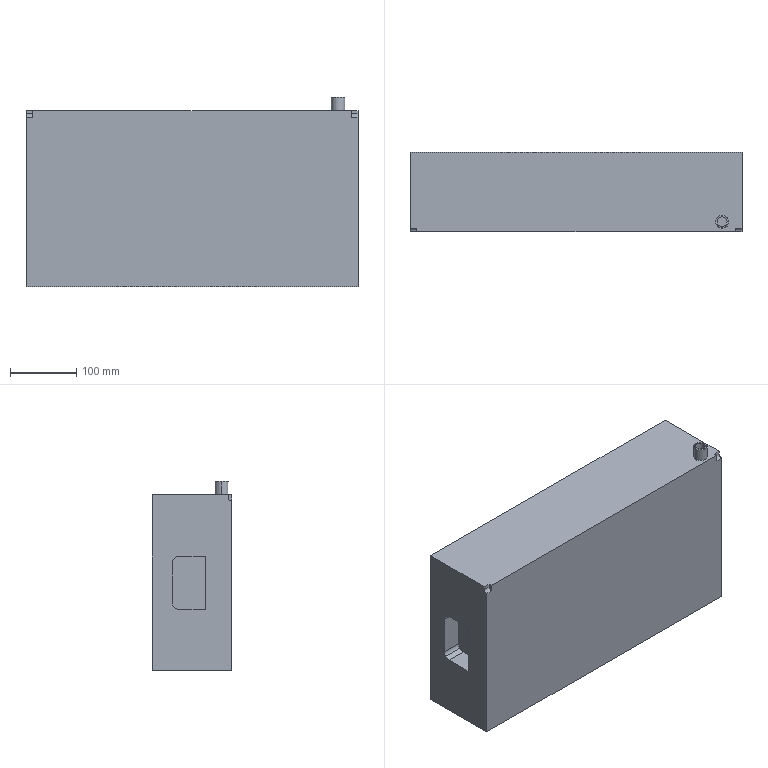Part | SolidWorks | features BaseBody 1 | 1 solid | 64 faces | box 500 x 120 x 285 mm | volume 1613110 mm3 | plane 38 | cylinder 24 | cone 2 | commonest cylinder face diameters 20 x12 30 x8 10 x2 15 x2